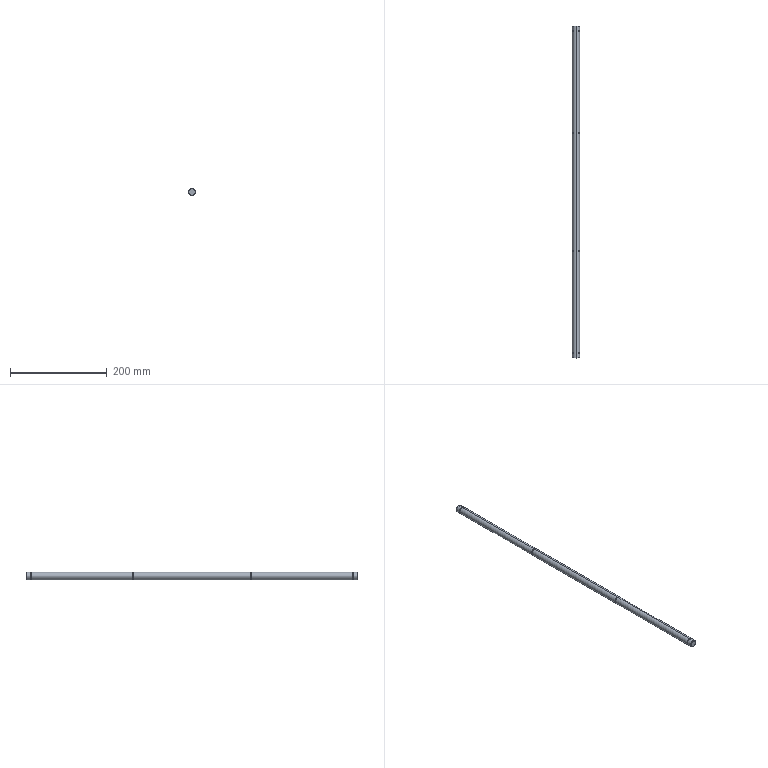Part | SolidWorks | features ICE 2, Chamfer 1, Extrusion 1, MirrorPattern 1 | 1 solid | 32 faces | box 15 x 688 x 15 mm | volume 121464 mm3 | cylinder 18 | plane 10 | cone 4 | commonest cylinder face diameters 15 x10 14.3 x8
STEP:
#1=CARTESIAN_POINT('',(0.,676.9,-7.5));
#2=VERTEX_POINT('',#1);
#3=CARTESIAN_POINT('',(0.,676.9,7.5));
#4=VERTEX_POINT('',#3);
#5=CARTESIAN_POINT('',(0.,676.9,0.));
#6=DIRECTION('',(0.,-1.,0.));
#7=DIRECTION('',(0.,0.,-1.));
#8=AXIS2_PLACEMENT_3D('',#5,#6,#7);
#9=CIRCLE('',#8,7.5);
#10=EDGE_CURVE('',#2,#4,#9,.T.);
#11=ORIENTED_EDGE('',*,*,#10,.T.);
#12=CARTESIAN_POINT('',(0.,467.,7.5));
#13=VERTEX_POINT('',#12);
#14=CARTESIAN_POINT('',(0.,688.,7.5));
#15=DIRECTION('',(0.,-1.,0.));
#16=VECTOR('',#15,1000.);
#17=LINE('',#14,#16);
#18=EDGE_CURVE('',#4,#13,#17,.T.);
#19=ORIENTED_EDGE('',*,*,#18,.T.);
#20=CARTESIAN_POINT('',(0.,467.,-7.5));
#21=VERTEX_POINT('',#20);
#22=CARTESIAN_POINT('',(0.,467.,0.));
#23=DIRECTION('',(0.,-1.,0.));
#24=DIRECTION('',(0.,0.,-1.));
#25=AXIS2_PLACEMENT_3D('',#22,#23,#24);
#26=CIRCLE('',#25,7.5);
#27=EDGE_CURVE('',#21,#13,#26,.T.);
#28=ORIENTED_EDGE('',*,*,#27,.F.);
#29=CARTESIAN_POINT('',(0.,688.,-7.5));
#30=DIRECTION('',(0.,-1.,0.));
#31=VECTOR('',#30,1000.);
#32=LINE('',#29,#31);
#33=EDGE_CURVE('',#2,#21,#32,.T.);
#34=ORIENTED_EDGE('',*,*,#33,.F.);
#35=EDGE_LOOP('',(#11,#19,#28,#34));
#36=FACE_OUTER_BOUND('',#35,.T.);
#37=CARTESIAN_POINT('',(0.,688.,0.));
#38=DIRECTION('',(0.,-1.,0.));
#39=DIRECTION('',(0.,0.,-1.));
#40=AXIS2_PLACEMENT_3D('',#37,#38,#39);
#41=CYLINDRICAL_SURFACE('',#40,7.5);
#42=ADVANCED_FACE('',(#36),#41,.T.);
#43=CARTESIAN_POINT('',(0.,676.9,-7.15));
#44=VERTEX_POINT('',#43);
#45=CARTESIAN_POINT('',(0.,676.9,7.15));
#46=VERTEX_POINT('',#45);
#47=CARTESIAN_POINT('',(0.,676.9,0.));
#48=DIRECTION('',(0.,-1.,0.));
#49=DIRECTION('',(0.,0.,-1.));
#50=AXIS2_PLACEMENT_3D('',#47,#48,#49);
#51=CIRCLE('',#50,7.15);
#52=EDGE_CURVE('',#44,#46,#51,.T.);
#53=ORIENTED_EDGE('',*,*,#52,.F.);
#54=CARTESIAN_POINT('',(0.,678.,-7.15));
#55=VERTEX_POINT('',#54);
#56=CARTESIAN_POINT('',(0.,676.9,-7.15));
#57=DIRECTION('',(0.,1.,0.));
#58=VECTOR('',#57,1000.);
#59=LINE('',#56,#58);
#60=EDGE_CURVE('',#44,#55,#59,.T.);
#61=ORIENTED_EDGE('',*,*,#60,.T.);
#62=CARTESIAN_POINT('',(0.,678.,7.15));
#63=VERTEX_POINT('',#62);
#64=CARTESIAN_POINT('',(0.,678.,0.));
#65=DIRECTION('',(0.,-1.,0.));
#66=DIRECTION('',(0.,0.,-1.));
#67=AXIS2_PLACEMENT_3D('',#64,#65,#66);
#68=CIRCLE('',#67,7.15);
#69=EDGE_CURVE('',#55,#63,#68,.T.);
#70=ORIENTED_EDGE('',*,*,#69,.T.);
#71=CARTESIAN_POINT('',(0.,676.9,7.15));
#72=DIRECTION('',(0.,1.,0.));
#73=VECTOR('',#72,1000.);
#74=LINE('',#71,#73);
#75=EDGE_CURVE('',#46,#63,#74,.T.);
#76=ORIENTED_EDGE('',*,*,#75,.F.);
#77=EDGE_LOOP('',(#53,#61,#70,#76));
#78=FACE_OUTER_BOUND('',#77,.T.);
#79=CARTESIAN_POINT('',(0.,676.9,0.));
#80=DIRECTION('',(0.,1.,0.));
#81=DIRECTION('',(0.,0.,1.));
#82=AXIS2_PLACEMENT_3D('',#79,#80,#81);
#83=CYLINDRICAL_SURFACE('',#82,7.15);
#84=ADVANCED_FACE('',(#78),#83,.T.);
#85=CARTESIAN_POINT('',(0.,687.,-7.5));
#86=VERTEX_POINT('',#85);
#87=CARTESIAN_POINT('',(0.,687.,7.5));
#88=VERTEX_POINT('',#87);
#89=CARTESIAN_POINT('',(0.,687.,0.));
#90=DIRECTION('',(0.,-1.,0.));
#91=DIRECTION('',(0.,0.,1.));
#92=AXIS2_PLACEMENT_3D('',#89,#90,#91);
#93=CIRCLE('',#92,7.5);
#94=EDGE_CURVE('',#86,#88,#93,.T.);
#95=ORIENTED_EDGE('',*,*,#94,.T.);
#96=CARTESIAN_POINT('',(0.,678.,7.5));
#97=VERTEX_POINT('',#96);
#98=CARTESIAN_POINT('',(0.,688.,7.5));
#99=DIRECTION('',(0.,-1.,0.));
#100=VECTOR('',#99,1000.);
#101=LINE('',#98,#100);
#102=EDGE_CURVE('',#88,#97,#101,.T.);
#103=ORIENTED_EDGE('',*,*,#102,.T.);
#104=CARTESIAN_POINT('',(0.,678.,-7.5));
#105=VERTEX_POINT('',#104);
#106=CARTESIAN_POINT('',(0.,678.,0.));
#107=DIRECTION('',(0.,-1.,0.));
#108=DIRECTION('',(0.,0.,-1.));
#109=AXIS2_PLACEMENT_3D('',#106,#107,#108);
#110=CIRCLE('',#109,7.5);
#111=EDGE_CURVE('',#105,#97,#110,.T.);
#112=ORIENTED_EDGE('',*,*,#111,.F.);
#113=CARTESIAN_POINT('',(0.,688.,-7.5));
#114=DIRECTION('',(0.,-1.,0.));
#115=VECTOR('',#114,1000.);
#116=LINE('',#113,#115);
#117=EDGE_CURVE('',#86,#105,#116,.T.);
#118=ORIENTED_EDGE('',*,*,#117,.F.);
#119=EDGE_LOOP('',(#95,#103,#112,#118));
#120=FACE_OUTER_BOUND('',#119,.T.);
#121=CARTESIAN_POINT('',(0.,688.,0.));
#122=DIRECTION('',(0.,-1.,0.));
#123=DIRECTION('',(0.,0.,-1.));
#124=AXIS2_PLACEMENT_3D('',#121,#122,#123);
#125=CYLINDRICAL_SURFACE('',#124,7.5);
#126=ADVANCED_FACE('',(#120),#125,.T.);
#127=CARTESIAN_POINT('',(0.,688.,6.5));
#128=VERTEX_POINT('',#127);
#129=CARTESIAN_POINT('',(0.,688.,-6.5));
#130=VERTEX_POINT('',#129);
#131=CARTESIAN_POINT('',(0.,688.,0.));
#132=DIRECTION('',(0.,1.,0.));
#133=DIRECTION('',(0.,0.,1.));
#134=AXIS2_PLACEMENT_3D('',#131,#132,#133);
#135=CIRCLE('',#134,6.5);
#136=EDGE_CURVE('',#128,#130,#135,.T.);
#137=ORIENTED_EDGE('',*,*,#136,.F.);
#138=CARTESIAN_POINT('',(0.,688.,6.5));
#139=DIRECTION('',(0.,-0.7071,0.7071));
#140=VECTOR('',#139,1000.);
#141=LINE('',#138,#140);
#142=EDGE_CURVE('',#128,#88,#141,.T.);
#143=ORIENTED_EDGE('',*,*,#142,.T.);
#144=ORIENTED_EDGE('',*,*,#94,.F.);
#145=CARTESIAN_POINT('',(0.,688.,-6.5));
#146=DIRECTION('',(0.,-0.7071,-0.7071));
#147=VECTOR('',#146,1000.);
#148=LINE('',#145,#147);
#149=EDGE_CURVE('',#130,#86,#148,.T.);
#150=ORIENTED_EDGE('',*,*,#149,.F.);
#151=EDGE_LOOP('',(#137,#143,#144,#150));
#152=FACE_OUTER_BOUND('',#151,.T.);
#153=CARTESIAN_POINT('',(0.,688.,0.));
#154=DIRECTION('',(0.,-1.,0.));
#155=DIRECTION('',(0.,0.,-1.));
#156=AXIS2_PLACEMENT_3D('',#153,#154,#155);
#157=CONICAL_SURFACE('',#156,6.5,0.7854);
#158=ADVANCED_FACE('',(#152),#157,.T.);
#159=CARTESIAN_POINT('',(0.,465.9,-7.15));
#160=VERTEX_POINT('',#159);
#161=CARTESIAN_POINT('',(0.,465.9,7.15));
#162=VERTEX_POINT('',#161);
#163=CARTESIAN_POINT('',(0.,465.9,0.));
#164=DIRECTION('',(0.,-1.,0.));
#165=DIRECTION('',(0.,0.,-1.));
#166=AXIS2_PLACEMENT_3D('',#163,#164,#165);
#167=CIRCLE('',#166,7.15);
#168=EDGE_CURVE('',#160,#162,#167,.T.);
#169=ORIENTED_EDGE('',*,*,#168,.F.);
#170=CARTESIAN_POINT('',(0.,467.,-7.15));
#171=VERTEX_POINT('',#170);
#172=CARTESIAN_POINT('',(0.,465.9,-7.15));
#173=DIRECTION('',(0.,1.,0.));
#174=VECTOR('',#173,1000.);
#175=LINE('',#172,#174);
#176=EDGE_CURVE('',#160,#171,#175,.T.);
#177=ORIENTED_EDGE('',*,*,#176,.T.);
#178=CARTESIAN_POINT('',(0.,467.,7.15));
#179=VERTEX_POINT('',#178);
#180=CARTESIAN_POINT('',(0.,467.,0.));
#181=DIRECTION('',(0.,-1.,0.));
#182=DIRECTION('',(0.,0.,-1.));
#183=AXIS2_PLACEMENT_3D('',#180,#181,#182);
#184=CIRCLE('',#183,7.15);
#185=EDGE_CURVE('',#171,#179,#184,.T.);
#186=ORIENTED_EDGE('',*,*,#185,.T.);
#187=CARTESIAN_POINT('',(0.,465.9,7.15));
#188=DIRECTION('',(0.,1.,0.));
#189=VECTOR('',#188,1000.);
#190=LINE('',#187,#189);
#191=EDGE_CURVE('',#162,#179,#190,.T.);
#192=ORIENTED_EDGE('',*,*,#191,.F.);
#193=EDGE_LOOP('',(#169,#177,#186,#192));
#194=FACE_OUTER_BOUND('',#193,.T.);
#195=CARTESIAN_POINT('',(0.,465.9,0.));
#196=DIRECTION('',(0.,1.,0.));
#197=DIRECTION('',(0.,0.,1.));
#198=AXIS2_PLACEMENT_3D('',#195,#196,#197);
#199=CYLINDRICAL_SURFACE('',#198,7.15);
#200=ADVANCED_FACE('',(#194),#199,.T.);
#201=CARTESIAN_POINT('',(0.,222.1,-7.15));
#202=VERTEX_POINT('',#201);
#203=CARTESIAN_POINT('',(0.,222.1,7.15));
#204=VERTEX_POINT('',#203);
#205=CARTESIAN_POINT('',(0.,222.1,0.));
#206=DIRECTION('',(0.,-1.,0.));
#207=DIRECTION('',(0.,0.,-1.));
#208=AXIS2_PLACEMENT_3D('',#205,#206,#207);
#209=CIRCLE('',#208,7.15);
#210=EDGE_CURVE('',#202,#204,#209,.T.);
#211=ORIENTED_EDGE('',*,*,#210,.T.);
#212=CARTESIAN_POINT('',(0.,221.,7.15));
#213=VERTEX_POINT('',#212);
#214=CARTESIAN_POINT('',(0.,222.1,7.15));
#215=DIRECTION('',(0.,-1.,0.));
#216=VECTOR('',#215,1000.);
#217=LINE('',#214,#216);
#218=EDGE_CURVE('',#204,#213,#217,.T.);
#219=ORIENTED_EDGE('',*,*,#218,.T.);
#220=CARTESIAN_POINT('',(0.,221.,-7.15));
#221=VERTEX_POINT('',#220);
#222=CARTESIAN_POINT('',(0.,221.,0.));
#223=DIRECTION('',(0.,-1.,0.));
#224=DIRECTION('',(0.,0.,-1.));
#225=AXIS2_PLACEMENT_3D('',#222,#223,#224);
#226=CIRCLE('',#225,7.15);
#227=EDGE_CURVE('',#221,#213,#226,.T.);
#228=ORIENTED_EDGE('',*,*,#227,.F.);
#229=CARTESIAN_POINT('',(0.,222.1,-7.15));
#230=DIRECTION('',(0.,-1.,0.));
#231=VECTOR('',#230,1000.);
#232=LINE('',#229,#231);
#233=EDGE_CURVE('',#202,#221,#232,.T.);
#234=ORIENTED_EDGE('',*,*,#233,.F.);
#235=EDGE_LOOP('',(#211,#219,#228,#234));
#236=FACE_OUTER_BOUND('',#235,.T.);
#237=CARTESIAN_POINT('',(0.,222.1,0.));
#238=DIRECTION('',(0.,-1.,0.));
#239=DIRECTION('',(0.,0.,-1.));
#240=AXIS2_PLACEMENT_3D('',#237,#238,#239);
#241=CYLINDRICAL_SURFACE('',#240,7.15);
#242=ADVANCED_FACE('',(#236),#241,.T.);
#243=CARTESIAN_POINT('',(0.,0.,-6.5));
#244=VERTEX_POINT('',#243);
#245=CARTESIAN_POINT('',(0.,0.,6.5));
#246=VERTEX_POINT('',#245);
#247=CARTESIAN_POINT('',(0.,0.,0.));
#248=DIRECTION('',(0.,-1.,0.));
#249=DIRECTION('',(0.,0.,1.));
#250=AXIS2_PLACEMENT_3D('',#247,#248,#249);
#251=CIRCLE('',#250,6.5);
#252=EDGE_CURVE('',#244,#246,#251,.T.);
#253=ORIENTED_EDGE('',*,*,#252,.F.);
#254=CARTESIAN_POINT('',(0.,1.,-7.5));
#255=VERTEX_POINT('',#254);
#256=CARTESIAN_POINT('',(0.,1.,-7.5));
#257=DIRECTION('',(0.,0.7071,-0.7071));
#258=VECTOR('',#257,1000.);
#259=LINE('',#256,#258);
#260=EDGE_CURVE('',#244,#255,#259,.T.);
#261=ORIENTED_EDGE('',*,*,#260,.T.);
#262=CARTESIAN_POINT('',(0.,1.,7.5));
#263=VERTEX_POINT('',#262);
#264=CARTESIAN_POINT('',(0.,1.,0.));
#265=DIRECTION('',(0.,1.,0.));
#266=DIRECTION('',(0.,0.,1.));
#267=AXIS2_PLACEMENT_3D('',#264,#265,#266);
#268=CIRCLE('',#267,7.5);
#269=EDGE_CURVE('',#263,#255,#268,.T.);
#270=ORIENTED_EDGE('',*,*,#269,.F.);
#271=CARTESIAN_POINT('',(0.,1.,7.5));
#272=DIRECTION('',(0.,0.7071,0.7071));
#273=VECTOR('',#272,1000.);
#274=LINE('',#271,#273);
#275=EDGE_CURVE('',#246,#263,#274,.T.);
#276=ORIENTED_EDGE('',*,*,#275,.F.);
#277=EDGE_LOOP('',(#253,#261,#270,#276));
#278=FACE_OUTER_BOUND('',#277,.T.);
#279=CARTESIAN_POINT('',(0.,1.,0.));
#280=DIRECTION('',(0.,1.,0.));
#281=DIRECTION('',(0.,0.,1.));
#282=AXIS2_PLACEMENT_3D('',#279,#280,#281);
#283=CONICAL_SURFACE('',#282,7.5,0.7854);
#284=ADVANCED_FACE('',(#278),#283,.T.);
#285=CARTESIAN_POINT('',(0.,10.,-7.5));
#286=VERTEX_POINT('',#285);
#287=CARTESIAN_POINT('',(0.,10.,7.5));
#288=VERTEX_POINT('',#287);
#289=CARTESIAN_POINT('',(0.,10.,0.));
#290=DIRECTION('',(0.,-1.,0.));
#291=DIRECTION('',(0.,0.,-1.));
#292=AXIS2_PLACEMENT_3D('',#289,#290,#291);
#293=CIRCLE('',#292,7.5);
#294=EDGE_CURVE('',#286,#288,#293,.T.);
#295=ORIENTED_EDGE('',*,*,#294,.T.);
#296=CARTESIAN_POINT('',(0.,688.,7.5));
#297=DIRECTION('',(0.,-1.,0.));
#298=VECTOR('',#297,1000.);
#299=LINE('',#296,#298);
#300=EDGE_CURVE('',#288,#263,#299,.T.);
#301=ORIENTED_EDGE('',*,*,#300,.T.);
#302=ORIENTED_EDGE('',*,*,#269,.T.);
#303=CARTESIAN_POINT('',(0.,688.,-7.5));
#304=DIRECTION('',(0.,-1.,0.));
#305=VECTOR('',#304,1000.);
#306=LINE('',#303,#305);
#307=EDGE_CURVE('',#286,#255,#306,.T.);
#308=ORIENTED_EDGE('',*,*,#307,.F.);
#309=EDGE_LOOP('',(#295,#301,#302,#308));
#310=FACE_OUTER_BOUND('',#309,.T.);
#311=CARTESIAN_POINT('',(0.,688.,0.));
#312=DIRECTION('',(0.,-1.,0.));
#313=DIRECTION('',(0.,0.,-1.));
#314=AXIS2_PLACEMENT_3D('',#311,#312,#313);
#315=CYLINDRICAL_SURFACE('',#314,7.5);
#316=ADVANCED_FACE('',(#310),#315,.T.);
#317=CARTESIAN_POINT('',(0.,11.1,-7.15));
#318=VERTEX_POINT('',#317);
#319=CARTESIAN_POINT('',(0.,11.1,7.15));
#320=VERTEX_POINT('',#319);
#321=CARTESIAN_POINT('',(0.,11.1,0.));
#322=DIRECTION('',(0.,-1.,0.));
#323=DIRECTION('',(0.,0.,-1.));
#324=AXIS2_PLACEMENT_3D('',#321,#322,#323);
#325=CIRCLE('',#324,7.15);
#326=EDGE_CURVE('',#318,#320,#325,.T.);
#327=ORIENTED_EDGE('',*,*,#326,.T.);
#328=CARTESIAN_POINT('',(0.,10.,7.15));
#329=VERTEX_POINT('',#328);
#330=CARTESIAN_POINT('',(0.,11.1,7.15));
#331=DIRECTION('',(0.,-1.,0.));
#332=VECTOR('',#331,1000.);
#333=LINE('',#330,#332);
#334=EDGE_CURVE('',#320,#329,#333,.T.);
#335=ORIENTED_EDGE('',*,*,#334,.T.);
#336=CARTESIAN_POINT('',(0.,10.,-7.15));
#337=VERTEX_POINT('',#336);
#338=CARTESIAN_POINT('',(0.,10.,0.));
#339=DIRECTION('',(0.,-1.,0.));
#340=DIRECTION('',(0.,0.,-1.));
#341=AXIS2_PLACEMENT_3D('',#338,#339,#340);
#342=CIRCLE('',#341,7.15);
#343=EDGE_CURVE('',#337,#329,#342,.T.);
#344=ORIENTED_EDGE('',*,*,#343,.F.);
#345=CARTESIAN_POINT('',(0.,11.1,-7.15));
#346=DIRECTION('',(0.,-1.,0.));
#347=VECTOR('',#346,1000.);
#348=LINE('',#345,#347);
#349=EDGE_CURVE('',#318,#337,#348,.T.);
#350=ORIENTED_EDGE('',*,*,#349,.F.);
#351=EDGE_LOOP('',(#327,#335,#344,#350));
#352=FACE_OUTER_BOUND('',#351,.T.);
#353=CARTESIAN_POINT('',(0.,11.1,0.));
#354=DIRECTION('',(0.,-1.,0.));
#355=DIRECTION('',(0.,0.,-1.));
#356=AXIS2_PLACEMENT_3D('',#353,#354,#355);
#357=CYLINDRICAL_SURFACE('',#356,7.15);
#358=ADVANCED_FACE('',(#352),#357,.T.);
#359=CARTESIAN_POINT('',(0.,221.,-7.5));
#360=VERTEX_POINT('',#359);
#361=CARTESIAN_POINT('',(0.,221.,7.5));
#362=VERTEX_POINT('',#361);
#363=CARTESIAN_POINT('',(0.,221.,0.));
#364=DIRECTION('',(0.,-1.,0.));
#365=DIRECTION('',(0.,0.,-1.));
#366=AXIS2_PLACEMENT_3D('',#363,#364,#365);
#367=CIRCLE('',#366,7.5);
#368=EDGE_CURVE('',#360,#362,#367,.T.);
#369=ORIENTED_EDGE('',*,*,#368,.T.);
#370=CARTESIAN_POINT('',(0.,11.1,7.5));
#371=VERTEX_POINT('',#370);
#372=CARTESIAN_POINT('',(0.,688.,7.5));
#373=DIRECTION('',(0.,-1.,0.));
#374=VECTOR('',#373,1000.);
#375=LINE('',#372,#374);
#376=EDGE_CURVE('',#362,#371,#375,.T.);
#377=ORIENTED_EDGE('',*,*,#376,.T.);
#378=CARTESIAN_POINT('',(0.,11.1,-7.5));
#379=VERTEX_POINT('',#378);
#380=CARTESIAN_POINT('',(0.,11.1,0.));
#381=DIRECTION('',(0.,-1.,0.));
#382=DIRECTION('',(0.,0.,-1.));
#383=AXIS2_PLACEMENT_3D('',#380,#381,#382);
#384=CIRCLE('',#383,7.5);
#385=EDGE_CURVE('',#379,#371,#384,.T.);
#386=ORIENTED_EDGE('',*,*,#385,.F.);
#387=CARTESIAN_POINT('',(0.,688.,-7.5));
#388=DIRECTION('',(0.,-1.,0.));
#389=VECTOR('',#388,1000.);
#390=LINE('',#387,#389);
#391=EDGE_CURVE('',#360,#379,#390,.T.);
#392=ORIENTED_EDGE('',*,*,#391,.F.);
#393=EDGE_LOOP('',(#369,#377,#386,#392));
#394=FACE_OUTER_BOUND('',#393,.T.);
#395=CARTESIAN_POINT('',(0.,688.,0.));
#396=DIRECTION('',(0.,-1.,0.));
#397=DIRECTION('',(0.,0.,-1.));
#398=AXIS2_PLACEMENT_3D('',#395,#396,#397);
#399=CYLINDRICAL_SURFACE('',#398,7.5);
#400=ADVANCED_FACE('',(#394),#399,.T.);
#401=CARTESIAN_POINT('',(0.,465.9,-7.5));
#402=VERTEX_POINT('',#401);
#403=CARTESIAN_POINT('',(0.,465.9,7.5));
#404=VERTEX_POINT('',#403);
#405=CARTESIAN_POINT('',(0.,465.9,0.));
#406=DIRECTION('',(0.,-1.,0.));
#407=DIRECTION('',(0.,0.,-1.));
#408=AXIS2_PLACEMENT_3D('',#405,#406,#407);
#409=CIRCLE('',#408,7.5);
#410=EDGE_CURVE('',#402,#404,#409,.T.);
#411=ORIENTED_EDGE('',*,*,#410,.T.);
#412=CARTESIAN_POINT('',(0.,222.1,7.5));
#413=VERTEX_POINT('',#412);
#414=CARTESIAN_POINT('',(0.,688.,7.5));
#415=DIRECTION('',(0.,-1.,0.));
#416=VECTOR('',#415,1000.);
#417=LINE('',#414,#416);
#418=EDGE_CURVE('',#404,#413,#417,.T.);
#419=ORIENTED_EDGE('',*,*,#418,.T.);
#420=CARTESIAN_POINT('',(0.,222.1,-7.5));
#421=VERTEX_POINT('',#420);
#422=CARTESIAN_POINT('',(0.,222.1,0.));
#423=DIRECTION('',(0.,-1.,0.));
#424=DIRECTION('',(0.,0.,-1.));
#425=AXIS2_PLACEMENT_3D('',#422,#423,#424);
#426=CIRCLE('',#425,7.5);
#427=EDGE_CURVE('',#421,#413,#426,.T.);
#428=ORIENTED_EDGE('',*,*,#427,.F.);
#429=CARTESIAN_POINT('',(0.,688.,-7.5));
#430=DIRECTION('',(0.,-1.,0.));
#431=VECTOR('',#430,1000.);
#432=LINE('',#429,#431);
#433=EDGE_CURVE('',#402,#421,#432,.T.);
#434=ORIENTED_EDGE('',*,*,#433,.F.);
#435=EDGE_LOOP('',(#411,#419,#428,#434));
#436=FACE_OUTER_BOUND('',#435,.T.);
#437=CARTESIAN_POINT('',(0.,688.,0.));
#438=DIRECTION('',(0.,-1.,0.));
#439=DIRECTION('',(0.,0.,-1.));
#440=AXIS2_PLACEMENT_3D('',#437,#438,#439);
#441=CYLINDRICAL_SURFACE('',#440,7.5);
#442=ADVANCED_FACE('',(#436),#441,.T.);
#443=ORIENTED_EDGE('',*,*,#418,.F.);
#444=CARTESIAN_POINT('',(0.,465.9,0.));
#445=DIRECTION('',(0.,-1.,0.));
#446=DIRECTION('',(0.,0.,-1.));
#447=AXIS2_PLACEMENT_3D('',#444,#445,#446);
#448=CIRCLE('',#447,7.5);
#449=EDGE_CURVE('',#404,#402,#448,.T.);
#450=ORIENTED_EDGE('',*,*,#449,.T.);
#451=ORIENTED_EDGE('',*,*,#433,.T.);
#452=CARTESIAN_POINT('',(0.,222.1,0.));
#453=DIRECTION('',(0.,-1.,0.));
#454=DIRECTION('',(0.,0.,-1.));
#455=AXIS2_PLACEMENT_3D('',#452,#453,#454);
#456=CIRCLE('',#455,7.5);
#457=EDGE_CURVE('',#413,#421,#456,.T.);
#458=ORIENTED_EDGE('',*,*,#457,.F.);
#459=EDGE_LOOP('',(#443,#450,#451,#458));
#460=FACE_OUTER_BOUND('',#459,.T.);
#461=CARTESIAN_POINT('',(0.,688.,0.));
#462=DIRECTION('',(0.,-1.,0.));
#463=DIRECTION('',(0.,0.,-1.));
#464=AXIS2_PLACEMENT_3D('',#461,#462,#463);
#465=CYLINDRICAL_SURFACE('',#464,7.5);
#466=ADVANCED_FACE('',(#460),#465,.T.);
#467=ORIENTED_EDGE('',*,*,#376,.F.);
#468=CARTESIAN_POINT('',(0.,221.,0.));
#469=DIRECTION('',(0.,-1.,0.));
#470=DIRECTION('',(0.,0.,-1.));
#471=AXIS2_PLACEMENT_3D('',#468,#469,#470);
#472=CIRCLE('',#471,7.5);
#473=EDGE_CURVE('',#362,#360,#472,.T.);
#474=ORIENTED_EDGE('',*,*,#473,.T.);
#475=ORIENTED_EDGE('',*,*,#391,.T.);
#476=CARTESIAN_POINT('',(0.,11.1,0.));
#477=DIRECTION('',(0.,-1.,0.));
#478=DIRECTION('',(0.,0.,-1.));
#479=AXIS2_PLACEMENT_3D('',#476,#477,#478);
#480=CIRCLE('',#479,7.5);
#481=EDGE_CURVE('',#371,#379,#480,.T.);
#482=ORIENTED_EDGE('',*,*,#481,.F.);
#483=EDGE_LOOP('',(#467,#474,#475,#482));
#484=FACE_OUTER_BOUND('',#483,.T.);
#485=CARTESIAN_POINT('',(0.,688.,0.));
#486=DIRECTION('',(0.,-1.,0.));
#487=DIRECTION('',(0.,0.,-1.));
#488=AXIS2_PLACEMENT_3D('',#485,#486,#487);
#489=CYLINDRICAL_SURFACE('',#488,7.5);
#490=ADVANCED_FACE('',(#484),#489,.T.);
#491=ORIENTED_EDGE('',*,*,#326,.F.);
#492=CARTESIAN_POINT('',(0.,11.1,0.));
#493=DIRECTION('',(0.,-1.,0.));
#494=DIRECTION('',(0.,0.,-1.));
#495=AXIS2_PLACEMENT_3D('',#492,#493,#494);
#496=CIRCLE('',#495,7.15);
#497=EDGE_CURVE('',#320,#318,#496,.T.);
#498=ORIENTED_EDGE('',*,*,#497,.F.);
#499=EDGE_LOOP('',(#491,#498));
#500=FACE_BOUND('',#499,.T.);
#501=ORIENTED_EDGE('',*,*,#385,.T.);
#502=ORIENTED_EDGE('',*,*,#481,.T.);
#503=EDGE_LOOP('',(#501,#502));
#504=FACE_OUTER_BOUND('',#503,.T.);
#505=CARTESIAN_POINT('',(0.,11.1,0.));
#506=DIRECTION('',(0.,-1.,0.));
#507=DIRECTION('',(0.,0.,-1.));
#508=AXIS2_PLACEMENT_3D('',#505,#506,#507);
#509=PLANE('',#508);
#510=ADVANCED_FACE('',(#500,#504),#509,.T.);
#511=ORIENTED_EDGE('',*,*,#343,.T.);
#512=CARTESIAN_POINT('',(0.,10.,0.));
#513=DIRECTION('',(0.,-1.,0.));
#514=DIRECTION('',(0.,0.,-1.));
#515=AXIS2_PLACEMENT_3D('',#512,#513,#514);
#516=CIRCLE('',#515,7.15);
#517=EDGE_CURVE('',#329,#337,#516,.T.);
#518=ORIENTED_EDGE('',*,*,#517,.T.);
#519=EDGE_LOOP('',(#511,#518));
#520=FACE_BOUND('',#519,.T.);
#521=ORIENTED_EDGE('',*,*,#294,.F.);
#522=CARTESIAN_POINT('',(0.,10.,0.));
#523=DIRECTION('',(0.,-1.,0.));
#524=DIRECTION('',(0.,0.,-1.));
#525=AXIS2_PLACEMENT_3D('',#522,#523,#524);
#526=CIRCLE('',#525,7.5);
#527=EDGE_CURVE('',#288,#286,#526,.T.);
#528=ORIENTED_EDGE('',*,*,#527,.F.);
#529=EDGE_LOOP('',(#521,#528));
#530=FACE_OUTER_BOUND('',#529,.T.);
#531=CARTESIAN_POINT('',(0.,10.,0.));
#532=DIRECTION('',(0.,-1.,0.));
#533=DIRECTION('',(0.,0.,-1.));
#534=AXIS2_PLACEMENT_3D('',#531,#532,#533);
#535=PLANE('',#534);
#536=ADVANCED_FACE('',(#520,#530),#535,.F.);
#537=ORIENTED_EDGE('',*,*,#334,.F.);
#538=ORIENTED_EDGE('',*,*,#497,.T.);
#539=ORIENTED_EDGE('',*,*,#349,.T.);
#540=ORIENTED_EDGE('',*,*,#517,.F.);
#541=EDGE_LOOP('',(#537,#538,#539,#540));
#542=FACE_OUTER_BOUND('',#541,.T.);
#543=CARTESIAN_POINT('',(0.,11.1,0.));
#544=DIRECTION('',(0.,-1.,0.));
#545=DIRECTION('',(0.,0.,-1.));
#546=AXIS2_PLACEMENT_3D('',#543,#544,#545);
#547=CYLINDRICAL_SURFACE('',#546,7.15);
#548=ADVANCED_FACE('',(#542),#547,.T.);
#549=CARTESIAN_POINT('',(0.,0.,0.));
#550=DIRECTION('',(0.,-1.,0.));
#551=DIRECTION('',(0.,0.,1.));
#552=AXIS2_PLACEMENT_3D('',#549,#550,#551);
#553=CIRCLE('',#552,6.5);
#554=EDGE_CURVE('',#246,#244,#553,.T.);
#555=ORIENTED_EDGE('',*,*,#554,.T.);
#556=ORIENTED_EDGE('',*,*,#252,.T.);
#557=EDGE_LOOP('',(#555,#556));
#558=FACE_OUTER_BOUND('',#557,.T.);
#559=CARTESIAN_POINT('',(0.,0.,0.));
#560=DIRECTION('',(0.,1.,0.));
#561=DIRECTION('',(0.,0.,1.));
#562=AXIS2_PLACEMENT_3D('',#559,#560,#561);
#563=PLANE('',#562);
#564=ADVANCED_FACE('',(#558),#563,.F.);
#565=ORIENTED_EDGE('',*,*,#300,.F.);
#566=ORIENTED_EDGE('',*,*,#527,.T.);
#567=ORIENTED_EDGE('',*,*,#307,.T.);
#568=CARTESIAN_POINT('',(0.,1.,0.));
#569=DIRECTION('',(0.,1.,0.));
#570=DIRECTION('',(0.,0.,1.));
#571=AXIS2_PLACEMENT_3D('',#568,#569,#570);
#572=CIRCLE('',#571,7.5);
#573=EDGE_CURVE('',#255,#263,#572,.T.);
#574=ORIENTED_EDGE('',*,*,#573,.T.);
#575=EDGE_LOOP('',(#565,#566,#567,#574));
#576=FACE_OUTER_BOUND('',#575,.T.);
#577=CARTESIAN_POINT('',(0.,688.,0.));
#578=DIRECTION('',(0.,-1.,0.));
#579=DIRECTION('',(0.,0.,-1.));
#580=AXIS2_PLACEMENT_3D('',#577,#578,#579);
#581=CYLINDRICAL_SURFACE('',#580,7.5);
#582=ADVANCED_FACE('',(#576),#581,.T.);
#583=ORIENTED_EDGE('',*,*,#260,.F.);
#584=ORIENTED_EDGE('',*,*,#554,.F.);
#585=ORIENTED_EDGE('',*,*,#275,.T.);
#586=ORIENTED_EDGE('',*,*,#573,.F.);
#587=EDGE_LOOP('',(#583,#584,#585,#586));
#588=FACE_OUTER_BOUND('',#587,.T.);
#589=CARTESIAN_POINT('',(0.,1.,0.));
#590=DIRECTION('',(0.,1.,0.));
#591=DIRECTION('',(0.,0.,1.));
#592=AXIS2_PLACEMENT_3D('',#589,#590,#591);
#593=CONICAL_SURFACE('',#592,7.5,0.7854);
#594=ADVANCED_FACE('',(#588),#593,.T.);
#595=ORIENTED_EDGE('',*,*,#210,.F.);
#596=CARTESIAN_POINT('',(0.,222.1,0.));
#597=DIRECTION('',(0.,-1.,0.));
#598=DIRECTION('',(0.,0.,-1.));
#599=AXIS2_PLACEMENT_3D('',#596,#597,#598);
#600=CIRCLE('',#599,7.15);
#601=EDGE_CURVE('',#204,#202,#600,.T.);
#602=ORIENTED_EDGE('',*,*,#601,.F.);
#603=EDGE_LOOP('',(#595,#602));
#604=FACE_BOUND('',#603,.T.);
#605=ORIENTED_EDGE('',*,*,#427,.T.);
#606=ORIENTED_EDGE('',*,*,#457,.T.);
#607=EDGE_LOOP('',(#605,#606));
#608=FACE_OUTER_BOUND('',#607,.T.);
#609=CARTESIAN_POINT('',(0.,222.1,0.));
#610=DIRECTION('',(0.,-1.,0.));
#611=DIRECTION('',(0.,0.,-1.));
#612=AXIS2_PLACEMENT_3D('',#609,#610,#611);
#613=PLANE('',#612);
#614=ADVANCED_FACE('',(#604,#608),#613,.T.);
#615=ORIENTED_EDGE('',*,*,#227,.T.);
#616=CARTESIAN_POINT('',(0.,221.,0.));
#617=DIRECTION('',(0.,-1.,0.));
#618=DIRECTION('',(0.,0.,-1.));
#619=AXIS2_PLACEMENT_3D('',#616,#617,#618);
#620=CIRCLE('',#619,7.15);
#621=EDGE_CURVE('',#213,#221,#620,.T.);
#622=ORIENTED_EDGE('',*,*,#621,.T.);
#623=EDGE_LOOP('',(#615,#622));
#624=FACE_BOUND('',#623,.T.);
#625=ORIENTED_EDGE('',*,*,#368,.F.);
#626=ORIENTED_EDGE('',*,*,#473,.F.);
#627=EDGE_LOOP('',(#625,#626));
#628=FACE_OUTER_BOUND('',#627,.T.);
#629=CARTESIAN_POINT('',(0.,221.,0.));
#630=DIRECTION('',(0.,-1.,0.));
#631=DIRECTION('',(0.,0.,-1.));
#632=AXIS2_PLACEMENT_3D('',#629,#630,#631);
#633=PLANE('',#632);
#634=ADVANCED_FACE('',(#624,#628),#633,.F.);
#635=ORIENTED_EDGE('',*,*,#218,.F.);
#636=ORIENTED_EDGE('',*,*,#601,.T.);
#637=ORIENTED_EDGE('',*,*,#233,.T.);
#638=ORIENTED_EDGE('',*,*,#621,.F.);
#639=EDGE_LOOP('',(#635,#636,#637,#638));
#640=FACE_OUTER_BOUND('',#639,.T.);
#641=CARTESIAN_POINT('',(0.,222.1,0.));
#642=DIRECTION('',(0.,-1.,0.));
#643=DIRECTION('',(0.,0.,-1.));
#644=AXIS2_PLACEMENT_3D('',#641,#642,#643);
#645=CYLINDRICAL_SURFACE('',#644,7.15);
#646=ADVANCED_FACE('',(#640),#645,.T.);
#647=ORIENTED_EDGE('',*,*,#410,.F.);
#648=ORIENTED_EDGE('',*,*,#449,.F.);
#649=EDGE_LOOP('',(#647,#648));
#650=FACE_OUTER_BOUND('',#649,.T.);
#651=CARTESIAN_POINT('',(0.,465.9,0.));
#652=DIRECTION('',(0.,-1.,0.));
#653=DIRECTION('',(0.,0.,-1.));
#654=AXIS2_PLACEMENT_3D('',#651,#652,#653);
#655=CIRCLE('',#654,7.15);
#656=EDGE_CURVE('',#162,#160,#655,.T.);
#657=ORIENTED_EDGE('',*,*,#656,.T.);
#658=ORIENTED_EDGE('',*,*,#168,.T.);
#659=EDGE_LOOP('',(#657,#658));
#660=FACE_BOUND('',#659,.T.);
#661=CARTESIAN_POINT('',(0.,465.9,0.));
#662=DIRECTION('',(0.,1.,0.));
#663=DIRECTION('',(0.,0.,-1.));
#664=AXIS2_PLACEMENT_3D('',#661,#662,#663);
#665=PLANE('',#664);
#666=ADVANCED_FACE('',(#650,#660),#665,.T.);
#667=ORIENTED_EDGE('',*,*,#27,.T.);
#668=CARTESIAN_POINT('',(0.,467.,0.));
#669=DIRECTION('',(0.,-1.,0.));
#670=DIRECTION('',(0.,0.,-1.));
#671=AXIS2_PLACEMENT_3D('',#668,#669,#670);
#672=CIRCLE('',#671,7.5);
#673=EDGE_CURVE('',#13,#21,#672,.T.);
#674=ORIENTED_EDGE('',*,*,#673,.T.);
#675=EDGE_LOOP('',(#667,#674));
#676=FACE_OUTER_BOUND('',#675,.T.);
#677=CARTESIAN_POINT('',(0.,467.,0.));
#678=DIRECTION('',(0.,-1.,0.));
#679=DIRECTION('',(0.,0.,-1.));
#680=AXIS2_PLACEMENT_3D('',#677,#678,#679);
#681=CIRCLE('',#680,7.15);
#682=EDGE_CURVE('',#179,#171,#681,.T.);
#683=ORIENTED_EDGE('',*,*,#682,.F.);
#684=ORIENTED_EDGE('',*,*,#185,.F.);
#685=EDGE_LOOP('',(#683,#684));
#686=FACE_BOUND('',#685,.T.);
#687=CARTESIAN_POINT('',(0.,467.,0.));
#688=DIRECTION('',(0.,1.,0.));
#689=DIRECTION('',(0.,0.,-1.));
#690=AXIS2_PLACEMENT_3D('',#687,#688,#689);
#691=PLANE('',#690);
#692=ADVANCED_FACE('',(#676,#686),#691,.F.);
#693=ORIENTED_EDGE('',*,*,#176,.F.);
#694=ORIENTED_EDGE('',*,*,#656,.F.);
#695=ORIENTED_EDGE('',*,*,#191,.T.);
#696=ORIENTED_EDGE('',*,*,#682,.T.);
#697=EDGE_LOOP('',(#693,#694,#695,#696));
#698=FACE_OUTER_BOUND('',#697,.T.);
#699=CARTESIAN_POINT('',(0.,465.9,0.));
#700=DIRECTION('',(0.,1.,0.));
#701=DIRECTION('',(0.,0.,1.));
#702=AXIS2_PLACEMENT_3D('',#699,#700,#701);
#703=CYLINDRICAL_SURFACE('',#702,7.15);
#704=ADVANCED_FACE('',(#698),#703,.T.);
#705=CARTESIAN_POINT('',(0.,688.,0.));
#706=DIRECTION('',(0.,1.,0.));
#707=DIRECTION('',(0.,0.,1.));
#708=AXIS2_PLACEMENT_3D('',#705,#706,#707);
#709=CIRCLE('',#708,6.5);
#710=EDGE_CURVE('',#130,#128,#709,.T.);
#711=ORIENTED_EDGE('',*,*,#710,.T.);
#712=ORIENTED_EDGE('',*,*,#136,.T.);
#713=EDGE_LOOP('',(#711,#712));
#714=FACE_OUTER_BOUND('',#713,.T.);
#715=CARTESIAN_POINT('',(0.,688.,0.));
#716=DIRECTION('',(0.,1.,0.));
#717=DIRECTION('',(0.,0.,1.));
#718=AXIS2_PLACEMENT_3D('',#715,#716,#717);
#719=PLANE('',#718);
#720=ADVANCED_FACE('',(#714),#719,.T.);
#721=ORIENTED_EDGE('',*,*,#142,.F.);
#722=ORIENTED_EDGE('',*,*,#710,.F.);
#723=ORIENTED_EDGE('',*,*,#149,.T.);
#724=CARTESIAN_POINT('',(0.,687.,0.));
#725=DIRECTION('',(0.,-1.,0.));
#726=DIRECTION('',(0.,0.,1.));
#727=AXIS2_PLACEMENT_3D('',#724,#725,#726);
#728=CIRCLE('',#727,7.5);
#729=EDGE_CURVE('',#88,#86,#728,.T.);
#730=ORIENTED_EDGE('',*,*,#729,.F.);
#731=EDGE_LOOP('',(#721,#722,#723,#730));
#732=FACE_OUTER_BOUND('',#731,.T.);
#733=CARTESIAN_POINT('',(0.,688.,0.));
#734=DIRECTION('',(0.,-1.,0.));
#735=DIRECTION('',(0.,0.,-1.));
#736=AXIS2_PLACEMENT_3D('',#733,#734,#735);
#737=CONICAL_SURFACE('',#736,6.5,0.7854);
#738=ADVANCED_FACE('',(#732),#737,.T.);
#739=ORIENTED_EDGE('',*,*,#102,.F.);
#740=ORIENTED_EDGE('',*,*,#729,.T.);
#741=ORIENTED_EDGE('',*,*,#117,.T.);
#742=CARTESIAN_POINT('',(0.,678.,0.));
#743=DIRECTION('',(0.,-1.,0.));
#744=DIRECTION('',(0.,0.,-1.));
#745=AXIS2_PLACEMENT_3D('',#742,#743,#744);
#746=CIRCLE('',#745,7.5);
#747=EDGE_CURVE('',#97,#105,#746,.T.);
#748=ORIENTED_EDGE('',*,*,#747,.F.);
#749=EDGE_LOOP('',(#739,#740,#741,#748));
#750=FACE_OUTER_BOUND('',#749,.T.);
#751=CARTESIAN_POINT('',(0.,688.,0.));
#752=DIRECTION('',(0.,-1.,0.));
#753=DIRECTION('',(0.,0.,-1.));
#754=AXIS2_PLACEMENT_3D('',#751,#752,#753);
#755=CYLINDRICAL_SURFACE('',#754,7.5);
#756=ADVANCED_FACE('',(#750),#755,.T.);
#757=ORIENTED_EDGE('',*,*,#111,.T.);
#758=ORIENTED_EDGE('',*,*,#747,.T.);
#759=EDGE_LOOP('',(#757,#758));
#760=FACE_OUTER_BOUND('',#759,.T.);
#761=CARTESIAN_POINT('',(0.,678.,0.));
#762=DIRECTION('',(0.,-1.,0.));
#763=DIRECTION('',(0.,0.,-1.));
#764=AXIS2_PLACEMENT_3D('',#761,#762,#763);
#765=CIRCLE('',#764,7.15);
#766=EDGE_CURVE('',#63,#55,#765,.T.);
#767=ORIENTED_EDGE('',*,*,#766,.F.);
#768=ORIENTED_EDGE('',*,*,#69,.F.);
#769=EDGE_LOOP('',(#767,#768));
#770=FACE_BOUND('',#769,.T.);
#771=CARTESIAN_POINT('',(0.,678.,0.));
#772=DIRECTION('',(0.,1.,0.));
#773=DIRECTION('',(0.,0.,-1.));
#774=AXIS2_PLACEMENT_3D('',#771,#772,#773);
#775=PLANE('',#774);
#776=ADVANCED_FACE('',(#760,#770),#775,.F.);
#777=ORIENTED_EDGE('',*,*,#60,.F.);
#778=CARTESIAN_POINT('',(0.,676.9,0.));
#779=DIRECTION('',(0.,-1.,0.));
#780=DIRECTION('',(0.,0.,-1.));
#781=AXIS2_PLACEMENT_3D('',#778,#779,#780);
#782=CIRCLE('',#781,7.15);
#783=EDGE_CURVE('',#46,#44,#782,.T.);
#784=ORIENTED_EDGE('',*,*,#783,.F.);
#785=ORIENTED_EDGE('',*,*,#75,.T.);
#786=ORIENTED_EDGE('',*,*,#766,.T.);
#787=EDGE_LOOP('',(#777,#784,#785,#786));
#788=FACE_OUTER_BOUND('',#787,.T.);
#789=CARTESIAN_POINT('',(0.,676.9,0.));
#790=DIRECTION('',(0.,1.,0.));
#791=DIRECTION('',(0.,0.,1.));
#792=AXIS2_PLACEMENT_3D('',#789,#790,#791);
#793=CYLINDRICAL_SURFACE('',#792,7.15);
#794=ADVANCED_FACE('',(#788),#793,.T.);
#795=ORIENTED_EDGE('',*,*,#10,.F.);
#796=CARTESIAN_POINT('',(0.,676.9,0.));
#797=DIRECTION('',(0.,-1.,0.));
#798=DIRECTION('',(0.,0.,-1.));
#799=AXIS2_PLACEMENT_3D('',#796,#797,#798);
#800=CIRCLE('',#799,7.5);
#801=EDGE_CURVE('',#4,#2,#800,.T.);
#802=ORIENTED_EDGE('',*,*,#801,.F.);
#803=EDGE_LOOP('',(#795,#802));
#804=FACE_OUTER_BOUND('',#803,.T.);
#805=ORIENTED_EDGE('',*,*,#783,.T.);
#806=ORIENTED_EDGE('',*,*,#52,.T.);
#807=EDGE_LOOP('',(#805,#806));
#808=FACE_BOUND('',#807,.T.);
#809=CARTESIAN_POINT('',(0.,676.9,0.));
#810=DIRECTION('',(0.,1.,0.));
#811=DIRECTION('',(0.,0.,-1.));
#812=AXIS2_PLACEMENT_3D('',#809,#810,#811);
#813=PLANE('',#812);
#814=ADVANCED_FACE('',(#804,#808),#813,.T.);
#815=ORIENTED_EDGE('',*,*,#18,.F.);
#816=ORIENTED_EDGE('',*,*,#801,.T.);
#817=ORIENTED_EDGE('',*,*,#33,.T.);
#818=ORIENTED_EDGE('',*,*,#673,.F.);
#819=EDGE_LOOP('',(#815,#816,#817,#818));
#820=FACE_OUTER_BOUND('',#819,.T.);
#821=CARTESIAN_POINT('',(0.,688.,0.));
#822=DIRECTION('',(0.,-1.,0.));
#823=DIRECTION('',(0.,0.,-1.));
#824=AXIS2_PLACEMENT_3D('',#821,#822,#823);
#825=CYLINDRICAL_SURFACE('',#824,7.5);
#826=ADVANCED_FACE('',(#820),#825,.T.);
#827=CLOSED_SHELL('',(#42,#84,#126,#158,#200,#242,#284,#316,#358,#400,#442,#466,#490,#510,#536,#548,#564,#582,#594,#614,#634,#646,#666,#692,#704,#720,#738,#756,#776,#794,#814,#826));
#828=MANIFOLD_SOLID_BREP('',#827);
#829=CARTESIAN_POINT('',(0.,0.,0.));
#830=DIRECTION('',(0.,0.,1.));
#831=DIRECTION('',(1.,0.,0.));
#832=AXIS2_PLACEMENT_3D('',#829,#830,#831);
#833=(LENGTH_UNIT()NAMED_UNIT(*)SI_UNIT(.MILLI.,.METRE.));
#834=UNCERTAINTY_MEASURE_WITH_UNIT(LENGTH_MEASURE(0.00001),#833,'','');
#835=(NAMED_UNIT(*)PLANE_ANGLE_UNIT()SI_UNIT($,.RADIAN.));
#836=(NAMED_UNIT(*)SI_UNIT($,.STERADIAN.)SOLID_ANGLE_UNIT());
#837=(GEOMETRIC_REPRESENTATION_CONTEXT(3)GLOBAL_UNCERTAINTY_ASSIGNED_CONTEXT((#834))GLOBAL_UNIT_ASSIGNED_CONTEXT((#833,#835,#836))REPRESENTATION_CONTEXT('',''));
#838=ADVANCED_BREP_SHAPE_REPRESENTATION('',(#828,#832),#837);